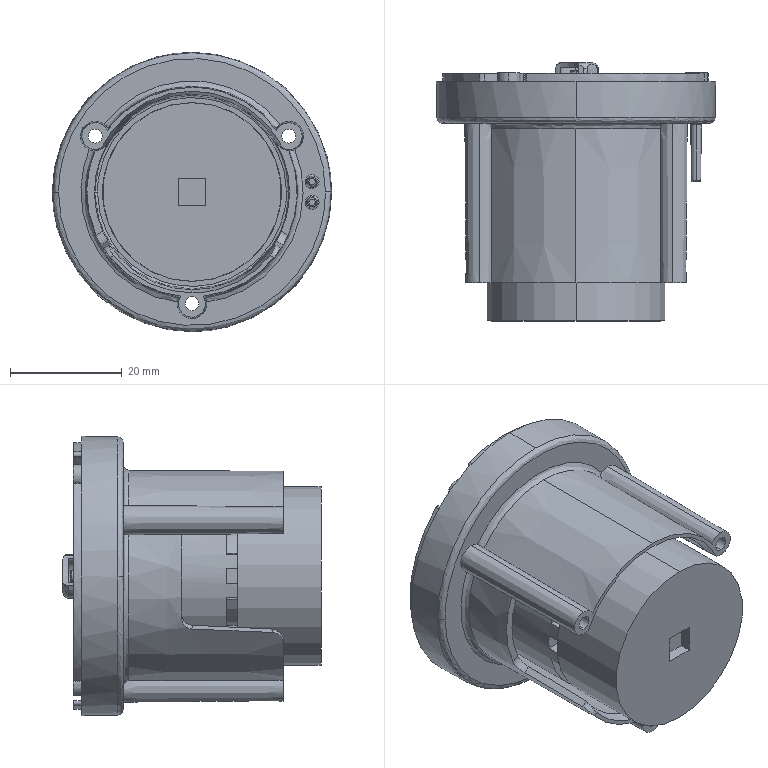Part | SolidWorks | features InContextFeatHolder 3 | 3 solids | 371 faces | box 50.005 x 46.2 x 50.005 mm | volume 37880 mm3 | plane 123 | cylinder 118 | cone 108 | spline 22 | commonest cylinder face diameters 4 x30 1.95 x10 1 x8 2 x8 2.8 x8 4.8 x8